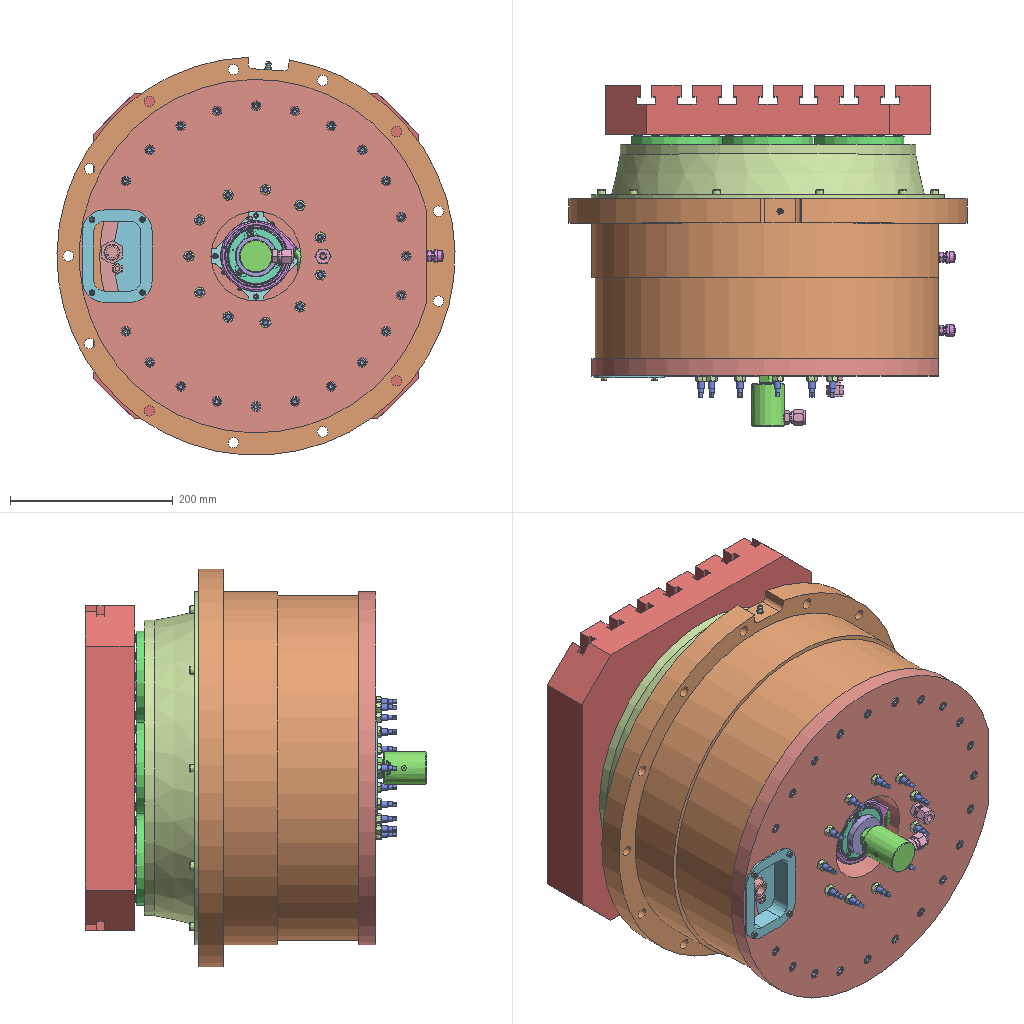Assembly | STEP file | 121 different items | 575 placed | box 490 x 420 x 489 mm
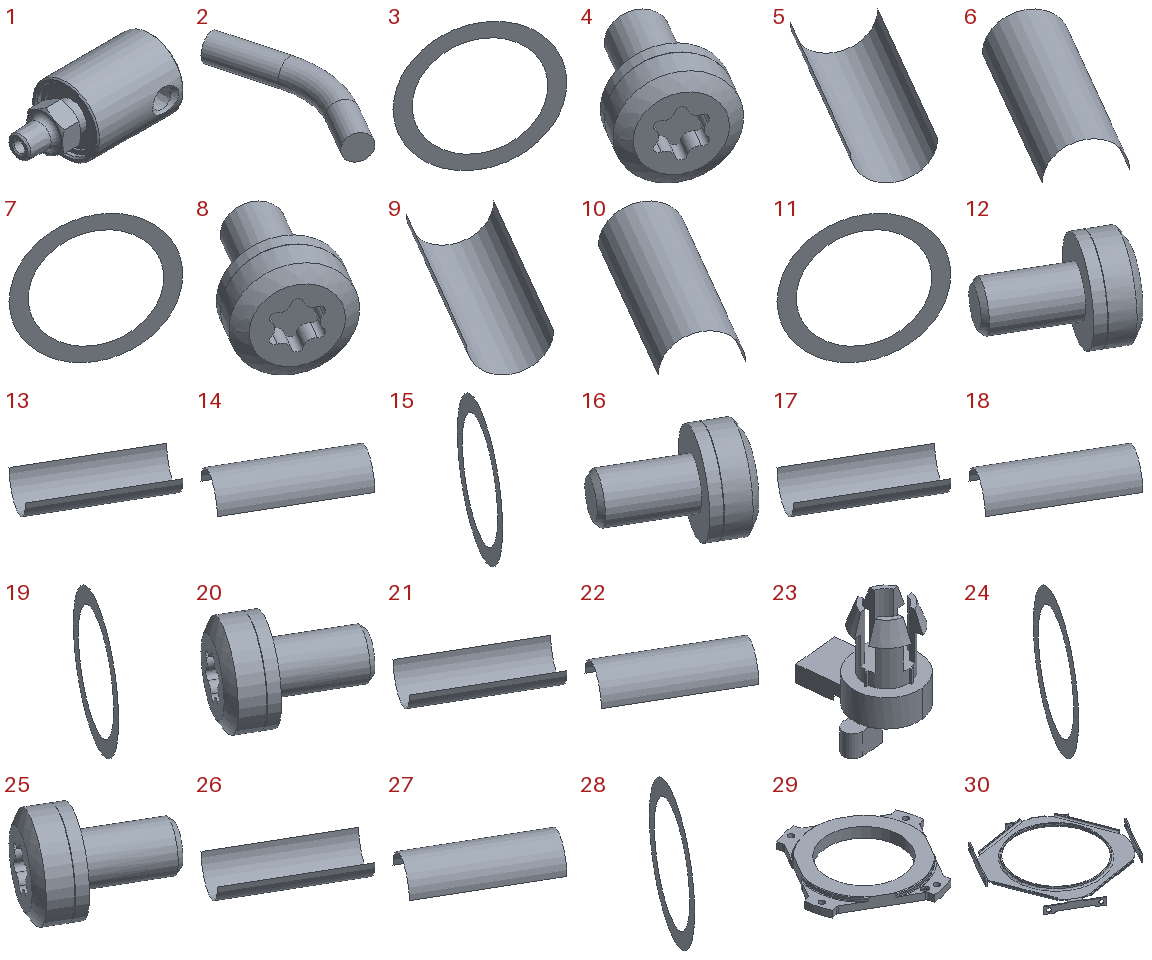Parts list (item | name | quantity | parent item | size | volume):
1 | 1102-070-082 | x1 | in Tilting rotary table | 80.735 x 40.71 x 40.71 mm | 70231 mm3
2 | - | x1 | in Encoder | 13.278 x 40.602 x 6 mm | 1151 mm3
3 | - | x1 | in Encoder | - | -
4 | - | x1 | in Encoder | 6.225 x 7.171 x 5 mm | 60.33 mm3
5 | - | x1 | in Encoder | - | -
6 | - | x1 | in Encoder | - | -
7 | - | x1 | in Encoder | - | -
8 | - | x1 | in Encoder | 6.225 x 7.171 x 5 mm | 60.33 mm3
9 | - | x1 | in Encoder | - | -
10 | - | x1 | in Encoder | - | -
11 | - | x1 | in Encoder | - | -
12 | - | x1 | in Encoder | 7.171 x 6.225 x 5 mm | 60.33 mm3
13 | - | x1 | in Encoder | - | -
14 | - | x1 | in Encoder | - | -
15 | - | x1 | in Encoder | - | -
16 | - | x1 | in Encoder | 7.171 x 6.225 x 5 mm | 60.33 mm3
17 | - | x1 | in Encoder | - | -
18 | - | x1 | in Encoder | - | -
19 | - | x1 | in Encoder | - | -
20 | - | x1 | in Encoder | 7.171 x 6.225 x 5 mm | 60.33 mm3
21 | - | x1 | in Encoder | - | -
22 | - | x1 | in Encoder | - | -
23 | - | x1 | in Encoder | 7.319 x 9.174 x 10 mm | 108.816 mm3
24 | - | x1 | in Encoder | - | -
25 | - | x1 | in Encoder | 7.171 x 6.225 x 5 mm | 60.33 mm3
26 | - | x1 | in Encoder | - | -
27 | - | x1 | in Encoder | - | -
28 | - | x1 | in Encoder | - | -
29 | - | x1 | in Encoder | 109.615 x 109.615 x 8.5 mm | 28096 mm3
30 | - | x1 | in Encoder | 90.075 x 84.017 x 12.5 mm | 2024 mm3
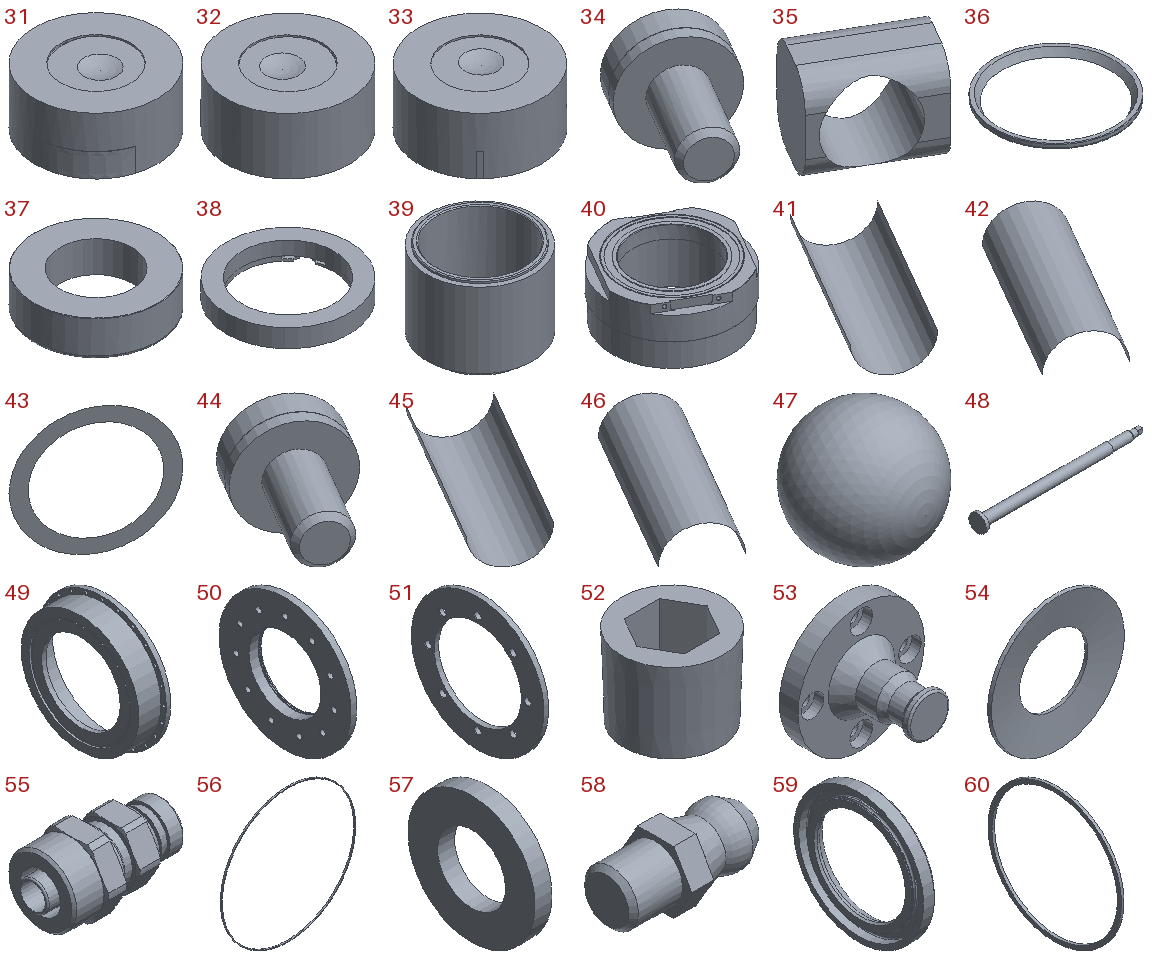31 | - | x1 | in Encoder | 7.6 x 7.6 x 4.3 mm | 142.649 mm3
32 | - | x1 | in Encoder | 7.6 x 7.622 x 4.3 mm | 142.648 mm3
33 | - | x1 | in Encoder | 7.618 x 7.6 x 4.3 mm | 142.649 mm3
34 | - | x1 | in Encoder | 6.225 x 7.171 x 5 mm | 60.33 mm3
35 | - | x1 | in Encoder | 10.188 x 9.346 x 7 mm | 153.66 mm3
36 | - | x1 | in Encoder | 78 x 78 x 4.5 mm | 2023 mm3
37 | - | x1 | in Encoder | 94.44 x 87 x 25 mm | 90953 mm3
38 | - | x1 | in Encoder | 67.8 x 67.8 x 10 mm | 15491 mm3
39 | - | x1 | in Encoder | 60 x 60 x 48 mm | 37487 mm3
40 | - | x1 | in Encoder | 87 x 87 x 39 mm | 122387 mm3
41 | - | x1 | in Encoder | - | -
42 | - | x1 | in Encoder | - | -
43 | - | x1 | in Encoder | - | -
44 | - | x1 | in Encoder | 6.225 x 7.171 x 5 mm | 60.33 mm3
45 | - | x1 | in Encoder | - | -
46 | - | x1 | in Encoder | - | -
47 | Ball | x19 | in Bearing 1000911 GOST 520-2011 | 7.5 x 7.5 x 7.5 mm | 220.893 mm3
48 | Bolt | x11 | in Tilting rotary table | 151 x 16 x 16 mm | 9327 mm3
49 | Brake disc | x1 | in Brake | 60 x 289 x 289 mm | 806797 mm3
50 | Brake half | x1 | in Brake | 20 x 220 x 220 mm | 280546 mm3
51 | Brake stopper | x1 | in Brake | 5 x 140 x 140 mm | 42146 mm3
52 | Cap | x9 | in Tilting rotary table | - | 438.849 mm3
53 | Clamping device rod | x4 | in Clamping device | 67.5 x 46.39 x 67.5 mm | 47194 mm3
54 | Disc spring | x154 | in Brake | 16 x 0.9 x 16 mm | 59.01 mm3
55 | Fitting | x2 | in Tilting rotary table | 26.3 x 15.5 x 14 mm | 2394 mm3
56 | Gasket | x2 | in Motor | 385 x 4 x 385 mm | 9626 mm3
57 | Gasket [2] | x4 | in Tilting rotary table | 2 x 15 x 15 mm | 252.898 mm3
58 | Grease nipple | x1 | in Tilting rotary table | 15.3 x 8.083 x 7 mm | 455.493 mm3
59 | Housing | x1 | in Cuff 1.1-55 x 80-1 / 4 GOST 8752-79 | 8 x 80 x 80 mm | 10893 mm3
60 | Inner gasket of clamping device | x4 | in Clamping device | 1 x 49.5 x 49.5 mm | 226.195 mm3
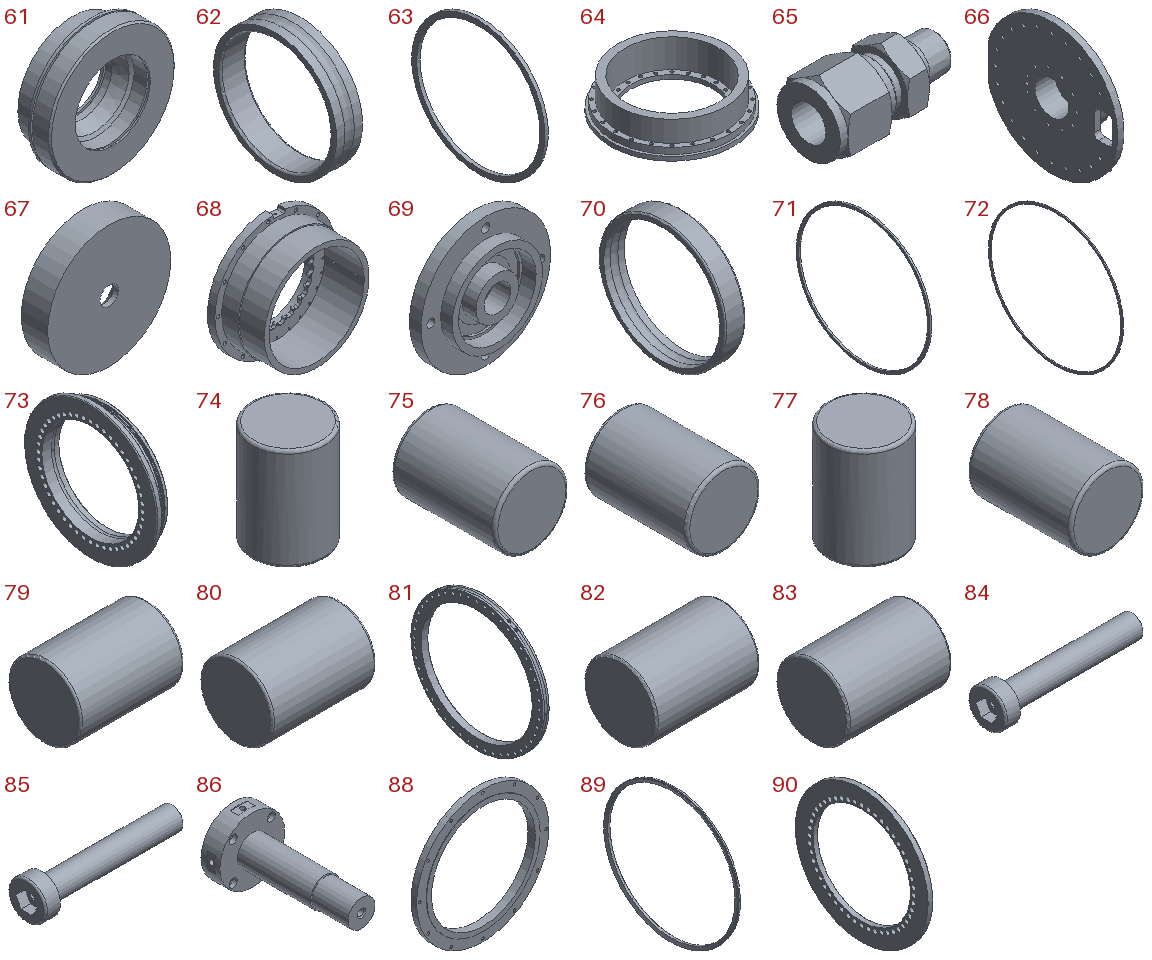61 | Inner part of clamp | x4 | in Clamping device | 78 x 25.32 x 78 mm | 67715 mm3
62 | Inner ring | x1 | in Bearing 1000911 GOST 520-2011 | 13 x 61.75 x 61.75 mm | 7419 mm3
63 | Inner seal of clamping device 2 | x4 | in Clamping device | 1 x 40 x 40 mm | 181.427 mm3
64 | Inner sleeve | x1 | in Tilting rotary table | 301 x 301 x 79.5 mm | 1463662 mm3
65 | LUMP1 | x2 | in Tilting rotary table | 35.052 x 17.463 x 20.164 mm | 4534 mm3
66 | Lower housing part | x1 | in Tilting rotary table | 109.5 x 427.5 x 435 mm | 4806369 mm3
67 | Lower part of clamping device | x4 | in Clamping device | 46.5 x 10 x 46.5 mm | 11861 mm3
68 | Outer housing | x1 | in Tilting rotary table | 490 x 197 x 489.832 mm | 8337866 mm3
69 | Outer part of clamping device | x4 | in Clamping device | 112 x 20 x 112 mm | 101943 mm3
70 | Outer ring | x1 | in Bearing 1000911 GOST 520-2011 | 13 x 80 x 80 mm | 9785 mm3
71 | Outer seal of clamping device | x4 | in Clamping device | 1 x 78 x 78 mm | 360.498 mm3
72 | Outer sealing ring | x2 | in Brake | 1 x 140 x 140 mm | 867.08 mm3
73 | Part | x1 | in Bearing | 34.993 x 274 x 274 mm | 543480 mm3
74 | Part [10] | x1 | in Bearing | 5 x 5 x 7 mm | 137.18 mm3
75 | Part [11] | x1 | in Bearing | 5 x 7 x 5 mm | 137.18 mm3
76 | Part [12] | x1 | in Bearing | 5 x 7 x 5 mm | 137.18 mm3
77 | Part [13] | x1 | in Bearing | 5 x 5 x 7 mm | 137.18 mm3
78 | Part [14] | x1 | in Bearing | 5 x 7 x 5 mm | 137.18 mm3
79 | Part [15] | x1 | in Bearing | 10 x 7 x 7 mm | 384.472 mm3
80 | Part [16] | x1 | in Bearing | 10 x 7 x 7 mm | 384.472 mm3
81 | Part [17] | x1 | in Bearing | 15 x 300 x 300 mm | 273448 mm3
82 | Part [18] | x1 | in Bearing | 10 x 7 x 7 mm | 384.472 mm3
83 | Part [19] | x1 | in Bearing | 10 x 7 x 7 mm | 384.472 mm3
84 | Part [20] | x1 | in Bearing | 39 x 10 x 10 mm | 1226 mm3
85 | Part [21] | x1 | in Bearing | 39 x 10 x 10 mm | 1226 mm3
86 | Part [22] | x1 | in Tilting rotary table | 120 x 247.5 x 120 mm | 802032 mm3
87 | Part [23] | x1 | in Tilting rotary table | - | -
88 | Part [24] | x1 | in Tilting rotary table | 350 x 24.5 x 350 mm | 570705 mm3
89 | Part [25] | x1 | in trelleborg_twvl03000-n6t50_bkreixb6isoqywg0uq1qlueij | 8 x 304.945 x 304.945 mm | 31163 mm3
90 | Part [2] | x1 | in Bearing | 10.03 x 274 x 274 mm | 241970 mm3
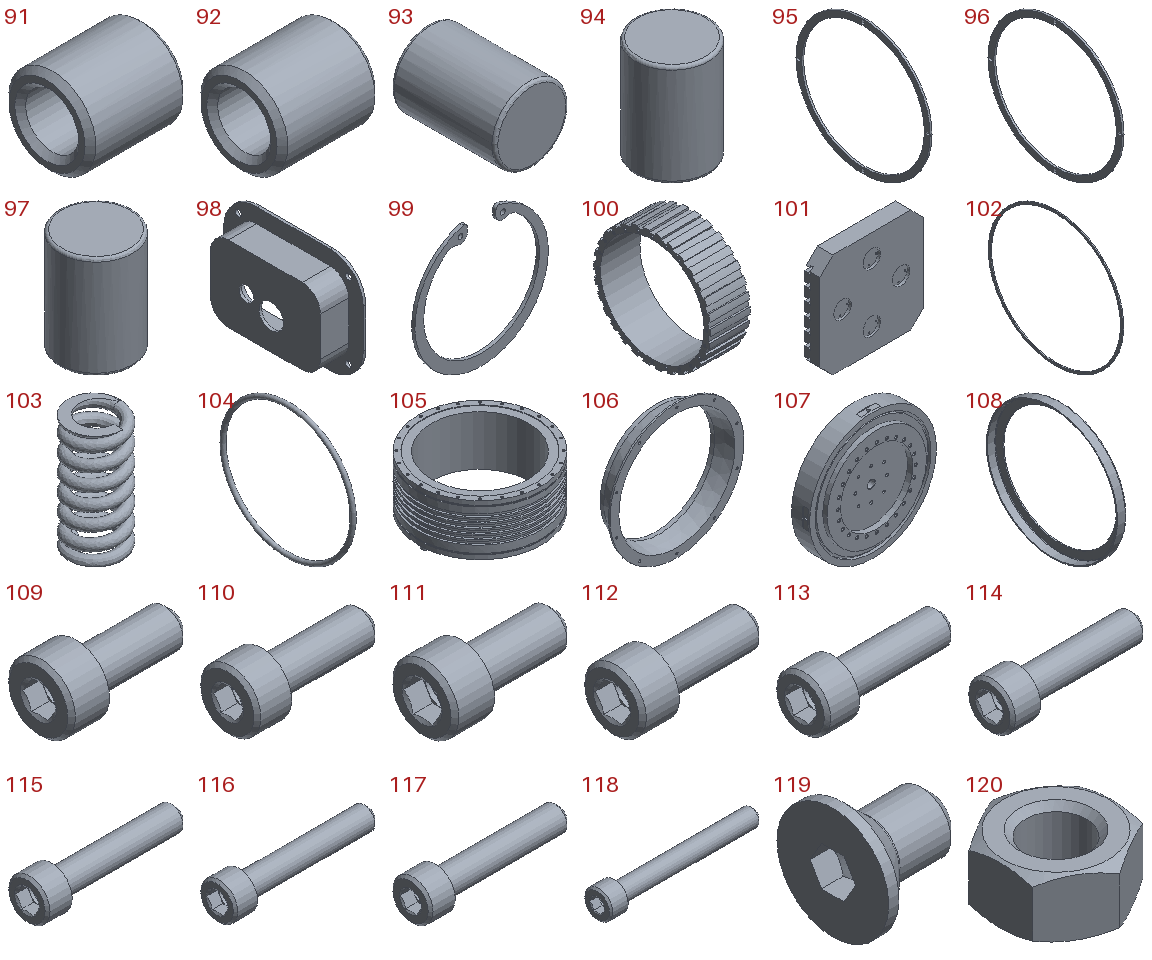91 | Part [3] | x1 | in Bearing | 9 x 8 x 8 mm | 272.983 mm3
92 | Part [4] | x1 | in Bearing | 9 x 8 x 8 mm | 272.983 mm3
93 | Part [5] | x1 | in Bearing | 5 x 7 x 5 mm | 137.18 mm3
94 | Part [6] | x1 | in Bearing | 5 x 5 x 7 mm | 137.18 mm3
95 | Part [7] | x1 | in Bearing | 4 x 272.1 x 272.1 mm | 37523 mm3
96 | Part [8] | x1 | in Bearing | 4 x 272.1 x 272.1 mm | 37523 mm3
97 | Part [9] | x1 | in Bearing | 5 x 5 x 7 mm | 137.18 mm3
98 | Plug | x1 | in Tilting rotary table | 25 x 114 x 86 mm | 29855 mm3
99 | Ring A80.65Г GOST 13943-86 | x1 | in Tilting rotary table | 83.5 x 2 x 81.948 mm | 2646 mm3
100 | Rotor | x1 | in Motor | 101 x 299 x 298.624 mm | 1274689 mm3
101 | Satellite table | x1 | in Tilting rotary table | 400 x 60 x 400 mm | 8025987 mm3
102 | Sealing ring | x2 | in Brake | 1 x 124 x 124 mm | 766.549 mm3
103 | Spring | x16 | in Clamping device | - | 251.261 mm3
104 | Spring [2] | x1 | in Cuff 1.1-55 x 80-1 / 4 GOST 8752-79 | 2.08 x 65.33 x 65.33 mm | 399.131 mm3
105 | Stator | x1 | in Motor | 385 x 385 x 173 mm | 6529567 mm3
106 | Upper cover | x1 | in Tilting rotary table | 435 x 67 x 435 mm | 550559 mm3
107 | Upper part | x1 | in Tilting rotary table | 350 x 60 x 350 mm | 4244226 mm3
108 | Valve | x1 | in Cuff 1.1-55 x 80-1 / 4 GOST 8752-79 | 5.28 x 77.925 x 77.925 mm | 1517 mm3
109 | Винт М4-6gx10 ГОСТ 11738-84 | x4 | in Tilting rotary table | 14 x 7 x 7 mm | 252.721 mm3
110 | Винт М4-6gx12 ГОСТ 11738-84 | x4 | in Tilting rotary table | 16 x 7 x 7 mm | 277.854 mm3
111 | Винт М6-6gx14 ГОСТ 11738-84 | x10 | in Tilting rotary table | 20 x 10 x 10 mm | 764.42 mm3
112 | Винт М6-6gx16 ГОСТ 11738-84 | x40 | in Tilting rotary table | 22 x 10 x 10 mm | 820.968 mm3
113 | Винт М6-6gx20 ГОСТ 11738-84 | x12 | in Tilting rotary table | 26 x 10 x 10 mm | 934.066 mm3
114 | Винт М6-6gx25 ГОСТ 11738-84 | x48 | in Tilting rotary table | 31 x 10 x 10 mm | 1075 mm3
115 | Винт М6-6gx30 ГОСТ 11738-84 | x45 | in Tilting rotary table | 36 x 10 x 10 mm | 1217 mm3
116 | Винт М6-6gx35 ГОСТ 11738-84 | x24 | in Tilting rotary table | 41 x 10 x 10 mm | 1358 mm3
117 | Винт М8-6gx40 ГОСТ 11738-84 | x4 | in Tilting rotary table | 48 x 13 x 13 mm | 2873 mm3
118 | Винт М8-6gx65 ГОСТ 11738-84 | x12 | in Tilting rotary table | 73 x 13 x 13 mm | 4129 mm3
119 | Винт с потайной головкой и шестигранным углублением под ключ ГОСТ Р ИСО 10642 - М6 x 10 - 8.8 | x4 | in Tilting rotary table | 10 x 11.34 x 11.34 mm | 400.146 mm3
120 | Гайка М8-6H ГОСТ 15521-70 | x11 | in Tilting rotary table | 12 x 13.856 x 6.5 mm | 565.148 mm3
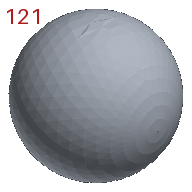121 | Шарик 12 мм | x16 | in Clamping device | 12 x 12 x 12 mm | 904.779 mm3